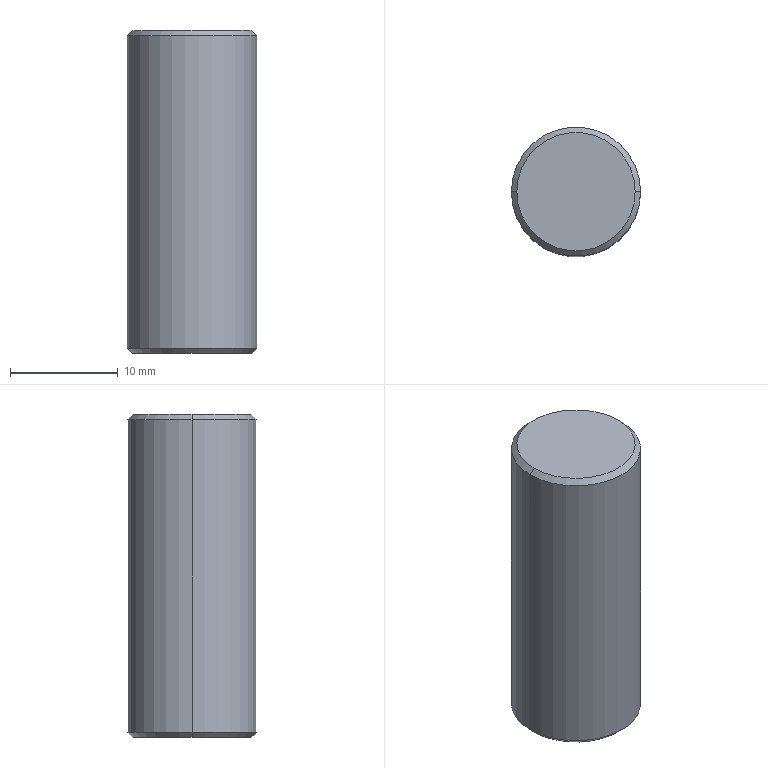Part | STEP file | 03-10 cylinder limit post | 1 solid | 12 faces | box 12 x 12 x 30 mm | volume 3278 mm3 | cone 6 | cylinder 4 | plane 2 | commonest cylinder face diameters 3.3 x2 12 x2
STEP:
#1=CARTESIAN_POINT('',(-5.5,0.,0.));
#2=VERTEX_POINT('',#1);
#3=CARTESIAN_POINT('',(5.5,0.,0.));
#4=VERTEX_POINT('',#3);
#5=CARTESIAN_POINT('',(0.,0.,0.));
#6=DIRECTION('',(0.,0.,-1.));
#7=DIRECTION('',(1.,0.,0.));
#8=AXIS2_PLACEMENT_3D('',#5,#6,#7);
#9=CIRCLE('',#8,5.5);
#10=EDGE_CURVE('',#2,#4,#9,.T.);
#11=ORIENTED_EDGE('',*,*,#10,.F.);
#12=CARTESIAN_POINT('',(-6.,0.,0.5));
#13=VERTEX_POINT('',#12);
#14=CARTESIAN_POINT('',(-6.,0.,0.5));
#15=DIRECTION('',(-0.7071,0.,0.7071));
#16=VECTOR('',#15,1000.);
#17=LINE('',#14,#16);
#18=EDGE_CURVE('',#2,#13,#17,.T.);
#19=ORIENTED_EDGE('',*,*,#18,.T.);
#20=CARTESIAN_POINT('',(6.,0.,0.5));
#21=VERTEX_POINT('',#20);
#22=CARTESIAN_POINT('',(0.,0.,0.5));
#23=DIRECTION('',(0.,0.,1.));
#24=DIRECTION('',(1.,0.,0.));
#25=AXIS2_PLACEMENT_3D('',#22,#23,#24);
#26=CIRCLE('',#25,6.);
#27=EDGE_CURVE('',#21,#13,#26,.T.);
#28=ORIENTED_EDGE('',*,*,#27,.F.);
#29=CARTESIAN_POINT('',(6.,0.,0.5));
#30=DIRECTION('',(0.7071,0.,0.7071));
#31=VECTOR('',#30,1000.);
#32=LINE('',#29,#31);
#33=EDGE_CURVE('',#4,#21,#32,.T.);
#34=ORIENTED_EDGE('',*,*,#33,.F.);
#35=EDGE_LOOP('',(#11,#19,#28,#34));
#36=FACE_OUTER_BOUND('',#35,.T.);
#37=CARTESIAN_POINT('',(0.,0.,0.5));
#38=DIRECTION('',(0.,0.,1.));
#39=DIRECTION('',(1.,0.,0.));
#40=AXIS2_PLACEMENT_3D('',#37,#38,#39);
#41=CONICAL_SURFACE('',#40,6.,0.7854);
#42=ADVANCED_FACE('',(#36),#41,.T.);
#43=CARTESIAN_POINT('',(5.5,0.,30.));
#44=VERTEX_POINT('',#43);
#45=CARTESIAN_POINT('',(-5.5,0.,30.));
#46=VERTEX_POINT('',#45);
#47=CARTESIAN_POINT('',(0.,0.,30.));
#48=DIRECTION('',(0.,0.,1.));
#49=DIRECTION('',(1.,0.,0.));
#50=AXIS2_PLACEMENT_3D('',#47,#48,#49);
#51=CIRCLE('',#50,5.5);
#52=EDGE_CURVE('',#44,#46,#51,.T.);
#53=ORIENTED_EDGE('',*,*,#52,.F.);
#54=CARTESIAN_POINT('',(6.,0.,29.5));
#55=VERTEX_POINT('',#54);
#56=CARTESIAN_POINT('',(5.5,0.,30.));
#57=DIRECTION('',(0.7071,0.,-0.7071));
#58=VECTOR('',#57,1000.);
#59=LINE('',#56,#58);
#60=EDGE_CURVE('',#44,#55,#59,.T.);
#61=ORIENTED_EDGE('',*,*,#60,.T.);
#62=CARTESIAN_POINT('',(-6.,0.,29.5));
#63=VERTEX_POINT('',#62);
#64=CARTESIAN_POINT('',(0.,0.,29.5));
#65=DIRECTION('',(0.,0.,-1.));
#66=DIRECTION('',(1.,0.,0.));
#67=AXIS2_PLACEMENT_3D('',#64,#65,#66);
#68=CIRCLE('',#67,6.);
#69=EDGE_CURVE('',#63,#55,#68,.T.);
#70=ORIENTED_EDGE('',*,*,#69,.F.);
#71=CARTESIAN_POINT('',(-5.5,0.,30.));
#72=DIRECTION('',(-0.7071,0.,-0.7071));
#73=VECTOR('',#72,1000.);
#74=LINE('',#71,#73);
#75=EDGE_CURVE('',#46,#63,#74,.T.);
#76=ORIENTED_EDGE('',*,*,#75,.F.);
#77=EDGE_LOOP('',(#53,#61,#70,#76));
#78=FACE_OUTER_BOUND('',#77,.T.);
#79=CARTESIAN_POINT('',(0.,0.,30.));
#80=DIRECTION('',(0.,0.,-1.));
#81=DIRECTION('',(-1.,0.,0.));
#82=AXIS2_PLACEMENT_3D('',#79,#80,#81);
#83=CONICAL_SURFACE('',#82,5.5,0.7854);
#84=ADVANCED_FACE('',(#78),#83,.T.);
#85=CARTESIAN_POINT('',(1.65,0.,12.));
#86=VERTEX_POINT('',#85);
#87=CARTESIAN_POINT('',(-1.65,0.,12.));
#88=VERTEX_POINT('',#87);
#89=CARTESIAN_POINT('',(0.,0.,12.));
#90=DIRECTION('',(0.,0.,-1.));
#91=DIRECTION('',(-1.,0.,0.));
#92=AXIS2_PLACEMENT_3D('',#89,#90,#91);
#93=CIRCLE('',#92,1.65);
#94=EDGE_CURVE('',#86,#88,#93,.T.);
#95=ORIENTED_EDGE('',*,*,#94,.F.);
#96=CARTESIAN_POINT('',(1.65,0.,0.));
#97=VERTEX_POINT('',#96);
#98=CARTESIAN_POINT('',(1.65,0.,0.));
#99=DIRECTION('',(0.,0.,-1.));
#100=VECTOR('',#99,1000.);
#101=LINE('',#98,#100);
#102=EDGE_CURVE('',#86,#97,#101,.T.);
#103=ORIENTED_EDGE('',*,*,#102,.T.);
#104=CARTESIAN_POINT('',(-1.65,0.,0.));
#105=VERTEX_POINT('',#104);
#106=CARTESIAN_POINT('',(0.,0.,0.));
#107=DIRECTION('',(0.,0.,-1.));
#108=DIRECTION('',(-1.,0.,0.));
#109=AXIS2_PLACEMENT_3D('',#106,#107,#108);
#110=CIRCLE('',#109,1.65);
#111=EDGE_CURVE('',#97,#105,#110,.T.);
#112=ORIENTED_EDGE('',*,*,#111,.T.);
#113=CARTESIAN_POINT('',(-1.65,0.,0.));
#114=DIRECTION('',(0.,0.,-1.));
#115=VECTOR('',#114,1000.);
#116=LINE('',#113,#115);
#117=EDGE_CURVE('',#88,#105,#116,.T.);
#118=ORIENTED_EDGE('',*,*,#117,.F.);
#119=EDGE_LOOP('',(#95,#103,#112,#118));
#120=FACE_OUTER_BOUND('',#119,.T.);
#121=CARTESIAN_POINT('',(0.,0.,0.));
#122=DIRECTION('',(0.,0.,-1.));
#123=DIRECTION('',(-1.,0.,0.));
#124=AXIS2_PLACEMENT_3D('',#121,#122,#123);
#125=CYLINDRICAL_SURFACE('',#124,1.65);
#126=ADVANCED_FACE('',(#120),#125,.F.);
#127=CARTESIAN_POINT('',(0.,0.,12.991));
#128=VERTEX_POINT('',#127);
#129=CARTESIAN_POINT('',(-1.65,0.,12.));
#130=DIRECTION('',(-0.8572,0.,-0.515));
#131=VECTOR('',#130,1000.);
#132=LINE('',#129,#131);
#133=EDGE_CURVE('',#128,#88,#132,.T.);
#134=ORIENTED_EDGE('',*,*,#133,.F.);
#135=CARTESIAN_POINT('',(1.65,0.,12.));
#136=DIRECTION('',(0.8572,0.,-0.515));
#137=VECTOR('',#136,1000.);
#138=LINE('',#135,#137);
#139=EDGE_CURVE('',#128,#86,#138,.T.);
#140=ORIENTED_EDGE('',*,*,#139,.T.);
#141=ORIENTED_EDGE('',*,*,#94,.T.);
#142=EDGE_LOOP('',(#134,#140,#141));
#143=FACE_OUTER_BOUND('',#142,.T.);
#144=CARTESIAN_POINT('',(0.,0.,12.));
#145=DIRECTION('',(0.,0.,-1.));
#146=DIRECTION('',(-1.,0.,0.));
#147=AXIS2_PLACEMENT_3D('',#144,#145,#146);
#148=CONICAL_SURFACE('',#147,1.65,1.03);
#149=ADVANCED_FACE('',(#143),#148,.F.);
#150=ORIENTED_EDGE('',*,*,#69,.T.);
#151=CARTESIAN_POINT('',(6.,0.,30.));
#152=DIRECTION('',(0.,0.,-1.));
#153=VECTOR('',#152,1000.);
#154=LINE('',#151,#153);
#155=EDGE_CURVE('',#55,#21,#154,.T.);
#156=ORIENTED_EDGE('',*,*,#155,.T.);
#157=ORIENTED_EDGE('',*,*,#27,.T.);
#158=CARTESIAN_POINT('',(-6.,0.,30.));
#159=DIRECTION('',(0.,0.,-1.));
#160=VECTOR('',#159,1000.);
#161=LINE('',#158,#160);
#162=EDGE_CURVE('',#63,#13,#161,.T.);
#163=ORIENTED_EDGE('',*,*,#162,.F.);
#164=EDGE_LOOP('',(#150,#156,#157,#163));
#165=FACE_OUTER_BOUND('',#164,.T.);
#166=CARTESIAN_POINT('',(0.,0.,30.));
#167=DIRECTION('',(0.,0.,-1.));
#168=DIRECTION('',(-1.,0.,0.));
#169=AXIS2_PLACEMENT_3D('',#166,#167,#168);
#170=CYLINDRICAL_SURFACE('',#169,6.);
#171=ADVANCED_FACE('',(#165),#170,.T.);
#172=ORIENTED_EDGE('',*,*,#155,.F.);
#173=CARTESIAN_POINT('',(0.,0.,29.5));
#174=DIRECTION('',(0.,0.,-1.));
#175=DIRECTION('',(1.,0.,0.));
#176=AXIS2_PLACEMENT_3D('',#173,#174,#175);
#177=CIRCLE('',#176,6.);
#178=EDGE_CURVE('',#55,#63,#177,.T.);
#179=ORIENTED_EDGE('',*,*,#178,.T.);
#180=ORIENTED_EDGE('',*,*,#162,.T.);
#181=CARTESIAN_POINT('',(0.,0.,0.5));
#182=DIRECTION('',(0.,0.,1.));
#183=DIRECTION('',(1.,0.,0.));
#184=AXIS2_PLACEMENT_3D('',#181,#182,#183);
#185=CIRCLE('',#184,6.);
#186=EDGE_CURVE('',#13,#21,#185,.T.);
#187=ORIENTED_EDGE('',*,*,#186,.T.);
#188=EDGE_LOOP('',(#172,#179,#180,#187));
#189=FACE_OUTER_BOUND('',#188,.T.);
#190=CARTESIAN_POINT('',(0.,0.,30.));
#191=DIRECTION('',(0.,0.,-1.));
#192=DIRECTION('',(-1.,0.,0.));
#193=AXIS2_PLACEMENT_3D('',#190,#191,#192);
#194=CYLINDRICAL_SURFACE('',#193,6.);
#195=ADVANCED_FACE('',(#189),#194,.T.);
#196=CARTESIAN_POINT('',(0.,0.,30.));
#197=DIRECTION('',(0.,0.,1.));
#198=DIRECTION('',(1.,0.,0.));
#199=AXIS2_PLACEMENT_3D('',#196,#197,#198);
#200=CIRCLE('',#199,5.5);
#201=EDGE_CURVE('',#46,#44,#200,.T.);
#202=ORIENTED_EDGE('',*,*,#201,.T.);
#203=ORIENTED_EDGE('',*,*,#52,.T.);
#204=EDGE_LOOP('',(#202,#203));
#205=FACE_OUTER_BOUND('',#204,.T.);
#206=CARTESIAN_POINT('',(0.,0.,30.));
#207=DIRECTION('',(0.,0.,1.));
#208=DIRECTION('',(1.,0.,0.));
#209=AXIS2_PLACEMENT_3D('',#206,#207,#208);
#210=PLANE('',#209);
#211=ADVANCED_FACE('',(#205),#210,.T.);
#212=CARTESIAN_POINT('',(0.,0.,0.));
#213=DIRECTION('',(0.,0.,-1.));
#214=DIRECTION('',(1.,0.,0.));
#215=AXIS2_PLACEMENT_3D('',#212,#213,#214);
#216=CIRCLE('',#215,5.5);
#217=EDGE_CURVE('',#4,#2,#216,.T.);
#218=ORIENTED_EDGE('',*,*,#217,.T.);
#219=ORIENTED_EDGE('',*,*,#10,.T.);
#220=EDGE_LOOP('',(#218,#219));
#221=FACE_OUTER_BOUND('',#220,.T.);
#222=CARTESIAN_POINT('',(0.,0.,0.));
#223=DIRECTION('',(0.,0.,-1.));
#224=DIRECTION('',(-1.,0.,0.));
#225=AXIS2_PLACEMENT_3D('',#222,#223,#224);
#226=CIRCLE('',#225,1.65);
#227=EDGE_CURVE('',#105,#97,#226,.T.);
#228=ORIENTED_EDGE('',*,*,#227,.F.);
#229=ORIENTED_EDGE('',*,*,#111,.F.);
#230=EDGE_LOOP('',(#228,#229));
#231=FACE_BOUND('',#230,.T.);
#232=CARTESIAN_POINT('',(0.,0.,0.));
#233=DIRECTION('',(0.,0.,1.));
#234=DIRECTION('',(1.,0.,0.));
#235=AXIS2_PLACEMENT_3D('',#232,#233,#234);
#236=PLANE('',#235);
#237=ADVANCED_FACE('',(#221,#231),#236,.F.);
#238=ORIENTED_EDGE('',*,*,#139,.F.);
#239=ORIENTED_EDGE('',*,*,#133,.T.);
#240=CARTESIAN_POINT('',(0.,0.,12.));
#241=DIRECTION('',(0.,0.,-1.));
#242=DIRECTION('',(-1.,0.,0.));
#243=AXIS2_PLACEMENT_3D('',#240,#241,#242);
#244=CIRCLE('',#243,1.65);
#245=EDGE_CURVE('',#88,#86,#244,.T.);
#246=ORIENTED_EDGE('',*,*,#245,.T.);
#247=EDGE_LOOP('',(#238,#239,#246));
#248=FACE_OUTER_BOUND('',#247,.T.);
#249=CARTESIAN_POINT('',(0.,0.,12.));
#250=DIRECTION('',(0.,0.,-1.));
#251=DIRECTION('',(-1.,0.,0.));
#252=AXIS2_PLACEMENT_3D('',#249,#250,#251);
#253=CONICAL_SURFACE('',#252,1.65,1.03);
#254=ADVANCED_FACE('',(#248),#253,.F.);
#255=ORIENTED_EDGE('',*,*,#102,.F.);
#256=ORIENTED_EDGE('',*,*,#245,.F.);
#257=ORIENTED_EDGE('',*,*,#117,.T.);
#258=ORIENTED_EDGE('',*,*,#227,.T.);
#259=EDGE_LOOP('',(#255,#256,#257,#258));
#260=FACE_OUTER_BOUND('',#259,.T.);
#261=CARTESIAN_POINT('',(0.,0.,0.));
#262=DIRECTION('',(0.,0.,-1.));
#263=DIRECTION('',(-1.,0.,0.));
#264=AXIS2_PLACEMENT_3D('',#261,#262,#263);
#265=CYLINDRICAL_SURFACE('',#264,1.65);
#266=ADVANCED_FACE('',(#260),#265,.F.);
#267=ORIENTED_EDGE('',*,*,#60,.F.);
#268=ORIENTED_EDGE('',*,*,#201,.F.);
#269=ORIENTED_EDGE('',*,*,#75,.T.);
#270=ORIENTED_EDGE('',*,*,#178,.F.);
#271=EDGE_LOOP('',(#267,#268,#269,#270));
#272=FACE_OUTER_BOUND('',#271,.T.);
#273=CARTESIAN_POINT('',(0.,0.,30.));
#274=DIRECTION('',(0.,0.,-1.));
#275=DIRECTION('',(-1.,0.,0.));
#276=AXIS2_PLACEMENT_3D('',#273,#274,#275);
#277=CONICAL_SURFACE('',#276,5.5,0.7854);
#278=ADVANCED_FACE('',(#272),#277,.T.);
#279=ORIENTED_EDGE('',*,*,#18,.F.);
#280=ORIENTED_EDGE('',*,*,#217,.F.);
#281=ORIENTED_EDGE('',*,*,#33,.T.);
#282=ORIENTED_EDGE('',*,*,#186,.F.);
#283=EDGE_LOOP('',(#279,#280,#281,#282));
#284=FACE_OUTER_BOUND('',#283,.T.);
#285=CARTESIAN_POINT('',(0.,0.,0.5));
#286=DIRECTION('',(0.,0.,1.));
#287=DIRECTION('',(1.,0.,0.));
#288=AXIS2_PLACEMENT_3D('',#285,#286,#287);
#289=CONICAL_SURFACE('',#288,6.,0.7854);
#290=ADVANCED_FACE('',(#284),#289,.T.);
#291=CLOSED_SHELL('',(#42,#84,#126,#149,#171,#195,#211,#237,#254,#266,#278,#290));
#292=MANIFOLD_SOLID_BREP('',#291);
#293=CARTESIAN_POINT('',(0.,0.,0.));
#294=DIRECTION('',(0.,0.,1.));
#295=DIRECTION('',(1.,0.,0.));
#296=AXIS2_PLACEMENT_3D('',#293,#294,#295);
#297=(LENGTH_UNIT()NAMED_UNIT(*)SI_UNIT(.MILLI.,.METRE.));
#298=UNCERTAINTY_MEASURE_WITH_UNIT(LENGTH_MEASURE(0.00001),#297,'','');
#299=(NAMED_UNIT(*)PLANE_ANGLE_UNIT()SI_UNIT($,.RADIAN.));
#300=(NAMED_UNIT(*)SI_UNIT($,.STERADIAN.)SOLID_ANGLE_UNIT());
#301=(GEOMETRIC_REPRESENTATION_CONTEXT(3)GLOBAL_UNCERTAINTY_ASSIGNED_CONTEXT((#298))GLOBAL_UNIT_ASSIGNED_CONTEXT((#297,#299,#300))REPRESENTATION_CONTEXT('',''));
#302=ADVANCED_BREP_SHAPE_REPRESENTATION('',(#292,#296),#301);